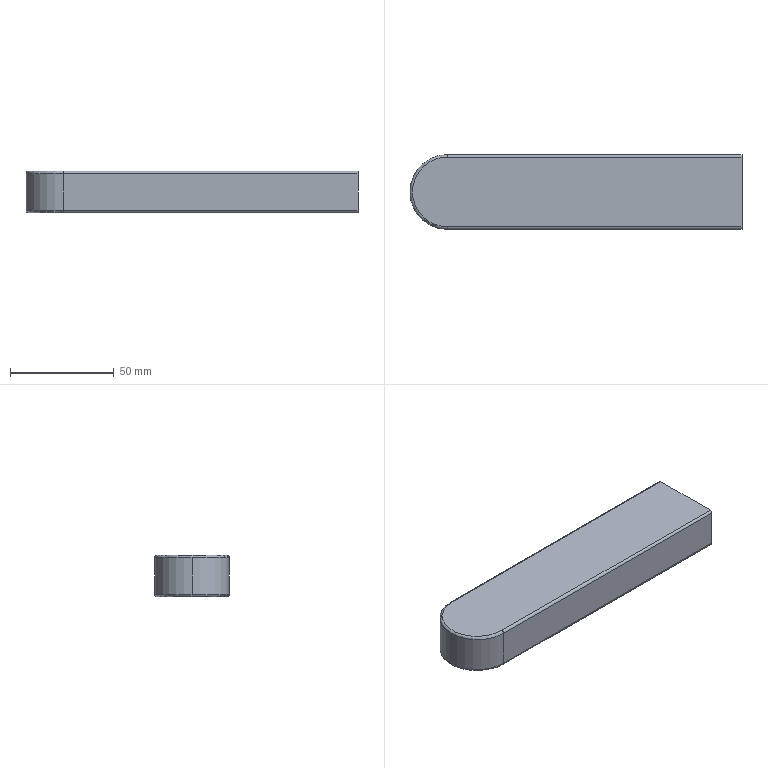Part | SolidWorks | features Extrusion 1, Fillet 1 | 1 solid | 13 faces | box 160 x 36 x 20 mm | volume 112209 mm3 | cylinder 6 | plane 5 | torus 2 | commonest cylinder face diameters 2.4 x4 36 x2
STEP:
#1=CARTESIAN_POINT('',(-9.,-18.,18.8));
#2=VERTEX_POINT('',#1);
#3=CARTESIAN_POINT('',(-27.,0.,18.8));
#4=VERTEX_POINT('',#3);
#5=CARTESIAN_POINT('',(-9.,0.,18.8));
#6=DIRECTION('',(0.,0.,-1.));
#7=DIRECTION('',(1.,0.,0.));
#8=AXIS2_PLACEMENT_3D('',#5,#6,#7);
#9=CIRCLE('',#8,18.);
#10=EDGE_CURVE('',#2,#4,#9,.T.);
#11=ORIENTED_EDGE('',*,*,#10,.T.);
#12=CARTESIAN_POINT('',(-27.,0.,1.2));
#13=VERTEX_POINT('',#12);
#14=CARTESIAN_POINT('',(-27.,0.,20.));
#15=DIRECTION('',(0.,0.,-1.));
#16=VECTOR('',#15,1000.);
#17=LINE('',#14,#16);
#18=EDGE_CURVE('',#4,#13,#17,.T.);
#19=ORIENTED_EDGE('',*,*,#18,.T.);
#20=CARTESIAN_POINT('',(-9.,-18.,1.2));
#21=VERTEX_POINT('',#20);
#22=CARTESIAN_POINT('',(-9.,0.,1.2));
#23=DIRECTION('',(0.,0.,1.));
#24=DIRECTION('',(1.,0.,0.));
#25=AXIS2_PLACEMENT_3D('',#22,#23,#24);
#26=CIRCLE('',#25,18.);
#27=EDGE_CURVE('',#13,#21,#26,.T.);
#28=ORIENTED_EDGE('',*,*,#27,.T.);
#29=CARTESIAN_POINT('',(-9.,-18.,20.));
#30=DIRECTION('',(0.,0.,-1.));
#31=VECTOR('',#30,1000.);
#32=LINE('',#29,#31);
#33=EDGE_CURVE('',#2,#21,#32,.T.);
#34=ORIENTED_EDGE('',*,*,#33,.F.);
#35=EDGE_LOOP('',(#11,#19,#28,#34));
#36=FACE_OUTER_BOUND('',#35,.T.);
#37=CARTESIAN_POINT('',(-9.,0.,20.));
#38=DIRECTION('',(0.,0.,-1.));
#39=DIRECTION('',(-1.,0.,0.));
#40=AXIS2_PLACEMENT_3D('',#37,#38,#39);
#41=CYLINDRICAL_SURFACE('',#40,18.);
#42=ADVANCED_FACE('',(#36),#41,.T.);
#43=CARTESIAN_POINT('',(133.,-16.8,20.));
#44=VERTEX_POINT('',#43);
#45=CARTESIAN_POINT('',(133.,16.8,20.));
#46=VERTEX_POINT('',#45);
#47=CARTESIAN_POINT('',(133.,18.,20.));
#48=DIRECTION('',(0.,1.,0.));
#49=VECTOR('',#48,1000.);
#50=LINE('',#47,#49);
#51=EDGE_CURVE('',#44,#46,#50,.T.);
#52=ORIENTED_EDGE('',*,*,#51,.F.);
#53=CARTESIAN_POINT('',(133.,-18.,18.8));
#54=VERTEX_POINT('',#53);
#55=CARTESIAN_POINT('',(133.,-16.8,18.8));
#56=DIRECTION('',(1.,0.,0.));
#57=DIRECTION('',(0.,0.,1.));
#58=AXIS2_PLACEMENT_3D('',#55,#56,#57);
#59=CIRCLE('',#58,1.2);
#60=EDGE_CURVE('',#44,#54,#59,.T.);
#61=ORIENTED_EDGE('',*,*,#60,.T.);
#62=CARTESIAN_POINT('',(133.,-18.,1.2));
#63=VERTEX_POINT('',#62);
#64=CARTESIAN_POINT('',(133.,-18.,20.));
#65=DIRECTION('',(0.,0.,-1.));
#66=VECTOR('',#65,1000.);
#67=LINE('',#64,#66);
#68=EDGE_CURVE('',#54,#63,#67,.T.);
#69=ORIENTED_EDGE('',*,*,#68,.T.);
#70=CARTESIAN_POINT('',(133.,-16.8,0.));
#71=VERTEX_POINT('',#70);
#72=CARTESIAN_POINT('',(133.,-16.8,1.2));
#73=DIRECTION('',(1.,0.,0.));
#74=DIRECTION('',(0.,0.,1.));
#75=AXIS2_PLACEMENT_3D('',#72,#73,#74);
#76=CIRCLE('',#75,1.2);
#77=EDGE_CURVE('',#63,#71,#76,.T.);
#78=ORIENTED_EDGE('',*,*,#77,.T.);
#79=CARTESIAN_POINT('',(133.,16.8,0.));
#80=VERTEX_POINT('',#79);
#81=CARTESIAN_POINT('',(133.,18.,0.));
#82=DIRECTION('',(0.,1.,0.));
#83=VECTOR('',#82,1000.);
#84=LINE('',#81,#83);
#85=EDGE_CURVE('',#71,#80,#84,.T.);
#86=ORIENTED_EDGE('',*,*,#85,.T.);
#87=CARTESIAN_POINT('',(133.,18.,1.2));
#88=VERTEX_POINT('',#87);
#89=CARTESIAN_POINT('',(133.,16.8,1.2));
#90=DIRECTION('',(1.,0.,0.));
#91=DIRECTION('',(0.,0.,1.));
#92=AXIS2_PLACEMENT_3D('',#89,#90,#91);
#93=CIRCLE('',#92,1.2);
#94=EDGE_CURVE('',#80,#88,#93,.T.);
#95=ORIENTED_EDGE('',*,*,#94,.T.);
#96=CARTESIAN_POINT('',(133.,18.,18.8));
#97=VERTEX_POINT('',#96);
#98=CARTESIAN_POINT('',(133.,18.,20.));
#99=DIRECTION('',(0.,0.,-1.));
#100=VECTOR('',#99,1000.);
#101=LINE('',#98,#100);
#102=EDGE_CURVE('',#97,#88,#101,.T.);
#103=ORIENTED_EDGE('',*,*,#102,.F.);
#104=CARTESIAN_POINT('',(133.,16.8,18.8));
#105=DIRECTION('',(1.,0.,0.));
#106=DIRECTION('',(0.,0.,1.));
#107=AXIS2_PLACEMENT_3D('',#104,#105,#106);
#108=CIRCLE('',#107,1.2);
#109=EDGE_CURVE('',#97,#46,#108,.T.);
#110=ORIENTED_EDGE('',*,*,#109,.T.);
#111=EDGE_LOOP('',(#52,#61,#69,#78,#86,#95,#103,#110));
#112=FACE_OUTER_BOUND('',#111,.T.);
#113=CARTESIAN_POINT('',(133.,18.,20.));
#114=DIRECTION('',(-1.,0.,0.));
#115=DIRECTION('',(0.,0.,1.));
#116=AXIS2_PLACEMENT_3D('',#113,#114,#115);
#117=PLANE('',#116);
#118=ADVANCED_FACE('',(#112),#117,.F.);
#119=CARTESIAN_POINT('',(-9.,18.,18.8));
#120=VERTEX_POINT('',#119);
#121=CARTESIAN_POINT('',(-9.,18.,1.2));
#122=VERTEX_POINT('',#121);
#123=CARTESIAN_POINT('',(-9.,18.,20.));
#124=DIRECTION('',(0.,0.,-1.));
#125=VECTOR('',#124,1000.);
#126=LINE('',#123,#125);
#127=EDGE_CURVE('',#120,#122,#126,.T.);
#128=ORIENTED_EDGE('',*,*,#127,.F.);
#129=CARTESIAN_POINT('',(133.,18.,18.8));
#130=DIRECTION('',(1.,0.,0.));
#131=VECTOR('',#130,1000.);
#132=LINE('',#129,#131);
#133=EDGE_CURVE('',#120,#97,#132,.T.);
#134=ORIENTED_EDGE('',*,*,#133,.T.);
#135=ORIENTED_EDGE('',*,*,#102,.T.);
#136=CARTESIAN_POINT('',(-9.,18.,1.2));
#137=DIRECTION('',(-1.,0.,0.));
#138=VECTOR('',#137,1000.);
#139=LINE('',#136,#138);
#140=EDGE_CURVE('',#88,#122,#139,.T.);
#141=ORIENTED_EDGE('',*,*,#140,.T.);
#142=EDGE_LOOP('',(#128,#134,#135,#141));
#143=FACE_OUTER_BOUND('',#142,.T.);
#144=CARTESIAN_POINT('',(-9.,18.,20.));
#145=DIRECTION('',(0.,-1.,0.));
#146=DIRECTION('',(0.,0.,-1.));
#147=AXIS2_PLACEMENT_3D('',#144,#145,#146);
#148=PLANE('',#147);
#149=ADVANCED_FACE('',(#143),#148,.F.);
#150=ORIENTED_EDGE('',*,*,#18,.F.);
#151=CARTESIAN_POINT('',(-9.,0.,18.8));
#152=DIRECTION('',(0.,0.,-1.));
#153=DIRECTION('',(1.,0.,0.));
#154=AXIS2_PLACEMENT_3D('',#151,#152,#153);
#155=CIRCLE('',#154,18.);
#156=EDGE_CURVE('',#4,#120,#155,.T.);
#157=ORIENTED_EDGE('',*,*,#156,.T.);
#158=ORIENTED_EDGE('',*,*,#127,.T.);
#159=CARTESIAN_POINT('',(-9.,0.,1.2));
#160=DIRECTION('',(0.,0.,1.));
#161=DIRECTION('',(1.,0.,0.));
#162=AXIS2_PLACEMENT_3D('',#159,#160,#161);
#163=CIRCLE('',#162,18.);
#164=EDGE_CURVE('',#122,#13,#163,.T.);
#165=ORIENTED_EDGE('',*,*,#164,.T.);
#166=EDGE_LOOP('',(#150,#157,#158,#165));
#167=FACE_OUTER_BOUND('',#166,.T.);
#168=CARTESIAN_POINT('',(-9.,0.,20.));
#169=DIRECTION('',(0.,0.,-1.));
#170=DIRECTION('',(-1.,0.,0.));
#171=AXIS2_PLACEMENT_3D('',#168,#169,#170);
#172=CYLINDRICAL_SURFACE('',#171,18.);
#173=ADVANCED_FACE('',(#167),#172,.T.);
#174=ORIENTED_EDGE('',*,*,#68,.F.);
#175=CARTESIAN_POINT('',(-9.,-18.,18.8));
#176=DIRECTION('',(-1.,0.,0.));
#177=VECTOR('',#176,1000.);
#178=LINE('',#175,#177);
#179=EDGE_CURVE('',#54,#2,#178,.T.);
#180=ORIENTED_EDGE('',*,*,#179,.T.);
#181=ORIENTED_EDGE('',*,*,#33,.T.);
#182=CARTESIAN_POINT('',(-9.,-18.,1.2));
#183=DIRECTION('',(1.,0.,0.));
#184=VECTOR('',#183,1000.);
#185=LINE('',#182,#184);
#186=EDGE_CURVE('',#21,#63,#185,.T.);
#187=ORIENTED_EDGE('',*,*,#186,.T.);
#188=EDGE_LOOP('',(#174,#180,#181,#187));
#189=FACE_OUTER_BOUND('',#188,.T.);
#190=CARTESIAN_POINT('',(-9.,-18.,20.));
#191=DIRECTION('',(0.,1.,0.));
#192=DIRECTION('',(0.,0.,1.));
#193=AXIS2_PLACEMENT_3D('',#190,#191,#192);
#194=PLANE('',#193);
#195=ADVANCED_FACE('',(#189),#194,.F.);
#196=CARTESIAN_POINT('',(-9.,16.8,20.));
#197=VERTEX_POINT('',#196);
#198=CARTESIAN_POINT('',(-9.,-16.8,20.));
#199=VERTEX_POINT('',#198);
#200=CARTESIAN_POINT('',(-9.,0.,20.));
#201=DIRECTION('',(0.,0.,1.));
#202=DIRECTION('',(1.,0.,0.));
#203=AXIS2_PLACEMENT_3D('',#200,#201,#202);
#204=CIRCLE('',#203,16.8);
#205=EDGE_CURVE('',#197,#199,#204,.T.);
#206=ORIENTED_EDGE('',*,*,#205,.T.);
#207=CARTESIAN_POINT('',(133.,-16.8,20.));
#208=DIRECTION('',(1.,0.,0.));
#209=VECTOR('',#208,1000.);
#210=LINE('',#207,#209);
#211=EDGE_CURVE('',#199,#44,#210,.T.);
#212=ORIENTED_EDGE('',*,*,#211,.T.);
#213=ORIENTED_EDGE('',*,*,#51,.T.);
#214=CARTESIAN_POINT('',(-9.,16.8,20.));
#215=DIRECTION('',(-1.,0.,0.));
#216=VECTOR('',#215,1000.);
#217=LINE('',#214,#216);
#218=EDGE_CURVE('',#46,#197,#217,.T.);
#219=ORIENTED_EDGE('',*,*,#218,.T.);
#220=EDGE_LOOP('',(#206,#212,#213,#219));
#221=FACE_OUTER_BOUND('',#220,.T.);
#222=CARTESIAN_POINT('',(-9.,0.,20.));
#223=DIRECTION('',(0.,0.,1.));
#224=DIRECTION('',(1.,0.,0.));
#225=AXIS2_PLACEMENT_3D('',#222,#223,#224);
#226=PLANE('',#225);
#227=ADVANCED_FACE('',(#221),#226,.T.);
#228=CARTESIAN_POINT('',(-9.,-16.8,0.));
#229=VERTEX_POINT('',#228);
#230=CARTESIAN_POINT('',(-9.,16.8,0.));
#231=VERTEX_POINT('',#230);
#232=CARTESIAN_POINT('',(-9.,0.,0.));
#233=DIRECTION('',(0.,0.,-1.));
#234=DIRECTION('',(1.,0.,0.));
#235=AXIS2_PLACEMENT_3D('',#232,#233,#234);
#236=CIRCLE('',#235,16.8);
#237=EDGE_CURVE('',#229,#231,#236,.T.);
#238=ORIENTED_EDGE('',*,*,#237,.T.);
#239=CARTESIAN_POINT('',(-9.,16.8,0.));
#240=DIRECTION('',(1.,0.,0.));
#241=VECTOR('',#240,1000.);
#242=LINE('',#239,#241);
#243=EDGE_CURVE('',#231,#80,#242,.T.);
#244=ORIENTED_EDGE('',*,*,#243,.T.);
#245=ORIENTED_EDGE('',*,*,#85,.F.);
#246=CARTESIAN_POINT('',(-9.,-16.8,0.));
#247=DIRECTION('',(-1.,0.,0.));
#248=VECTOR('',#247,1000.);
#249=LINE('',#246,#248);
#250=EDGE_CURVE('',#71,#229,#249,.T.);
#251=ORIENTED_EDGE('',*,*,#250,.T.);
#252=EDGE_LOOP('',(#238,#244,#245,#251));
#253=FACE_OUTER_BOUND('',#252,.T.);
#254=CARTESIAN_POINT('',(-9.,0.,0.));
#255=DIRECTION('',(0.,0.,1.));
#256=DIRECTION('',(1.,0.,0.));
#257=AXIS2_PLACEMENT_3D('',#254,#255,#256);
#258=PLANE('',#257);
#259=ADVANCED_FACE('',(#253),#258,.F.);
#260=ORIENTED_EDGE('',*,*,#109,.F.);
#261=ORIENTED_EDGE('',*,*,#133,.F.);
#262=CARTESIAN_POINT('',(-9.,16.8,18.8));
#263=DIRECTION('',(-1.,0.,0.));
#264=DIRECTION('',(0.,0.,1.));
#265=AXIS2_PLACEMENT_3D('',#262,#263,#264);
#266=CIRCLE('',#265,1.2);
#267=EDGE_CURVE('',#197,#120,#266,.T.);
#268=ORIENTED_EDGE('',*,*,#267,.F.);
#269=ORIENTED_EDGE('',*,*,#218,.F.);
#270=EDGE_LOOP('',(#260,#261,#268,#269));
#271=FACE_OUTER_BOUND('',#270,.T.);
#272=CARTESIAN_POINT('',(-9.,16.8,18.8));
#273=DIRECTION('',(1.,0.,0.));
#274=DIRECTION('',(0.,0.,-1.));
#275=AXIS2_PLACEMENT_3D('',#272,#273,#274);
#276=CYLINDRICAL_SURFACE('',#275,1.2);
#277=ADVANCED_FACE('',(#271),#276,.T.);
#278=ORIENTED_EDGE('',*,*,#267,.T.);
#279=ORIENTED_EDGE('',*,*,#156,.F.);
#280=ORIENTED_EDGE('',*,*,#10,.F.);
#281=CARTESIAN_POINT('',(-9.,-16.8,18.8));
#282=DIRECTION('',(1.,0.,0.));
#283=DIRECTION('',(0.,0.,-1.));
#284=AXIS2_PLACEMENT_3D('',#281,#282,#283);
#285=CIRCLE('',#284,1.2);
#286=EDGE_CURVE('',#199,#2,#285,.T.);
#287=ORIENTED_EDGE('',*,*,#286,.F.);
#288=ORIENTED_EDGE('',*,*,#205,.F.);
#289=EDGE_LOOP('',(#278,#279,#280,#287,#288));
#290=FACE_OUTER_BOUND('',#289,.T.);
#291=CARTESIAN_POINT('',(-9.,0.,18.8));
#292=DIRECTION('',(0.,0.,1.));
#293=DIRECTION('',(1.,0.,0.));
#294=AXIS2_PLACEMENT_3D('',#291,#292,#293);
#295=TOROIDAL_SURFACE('',#294,16.8,1.2);
#296=ADVANCED_FACE('',(#290),#295,.T.);
#297=ORIENTED_EDGE('',*,*,#286,.T.);
#298=ORIENTED_EDGE('',*,*,#179,.F.);
#299=ORIENTED_EDGE('',*,*,#60,.F.);
#300=ORIENTED_EDGE('',*,*,#211,.F.);
#301=EDGE_LOOP('',(#297,#298,#299,#300));
#302=FACE_OUTER_BOUND('',#301,.T.);
#303=CARTESIAN_POINT('',(-9.,-16.8,18.8));
#304=DIRECTION('',(-1.,0.,0.));
#305=DIRECTION('',(0.,0.,1.));
#306=AXIS2_PLACEMENT_3D('',#303,#304,#305);
#307=CYLINDRICAL_SURFACE('',#306,1.2);
#308=ADVANCED_FACE('',(#302),#307,.T.);
#309=ORIENTED_EDGE('',*,*,#77,.F.);
#310=ORIENTED_EDGE('',*,*,#186,.F.);
#311=CARTESIAN_POINT('',(-9.,-16.8,1.2));
#312=DIRECTION('',(-1.,0.,0.));
#313=DIRECTION('',(0.,0.,1.));
#314=AXIS2_PLACEMENT_3D('',#311,#312,#313);
#315=CIRCLE('',#314,1.2);
#316=EDGE_CURVE('',#229,#21,#315,.T.);
#317=ORIENTED_EDGE('',*,*,#316,.F.);
#318=ORIENTED_EDGE('',*,*,#250,.F.);
#319=EDGE_LOOP('',(#309,#310,#317,#318));
#320=FACE_OUTER_BOUND('',#319,.T.);
#321=CARTESIAN_POINT('',(-9.,-16.8,1.2));
#322=DIRECTION('',(1.,0.,0.));
#323=DIRECTION('',(0.,0.,-1.));
#324=AXIS2_PLACEMENT_3D('',#321,#322,#323);
#325=CYLINDRICAL_SURFACE('',#324,1.2);
#326=ADVANCED_FACE('',(#320),#325,.T.);
#327=ORIENTED_EDGE('',*,*,#316,.T.);
#328=ORIENTED_EDGE('',*,*,#27,.F.);
#329=ORIENTED_EDGE('',*,*,#164,.F.);
#330=CARTESIAN_POINT('',(-9.,16.8,1.2));
#331=DIRECTION('',(1.,0.,0.));
#332=DIRECTION('',(0.,0.,-1.));
#333=AXIS2_PLACEMENT_3D('',#330,#331,#332);
#334=CIRCLE('',#333,1.2);
#335=EDGE_CURVE('',#231,#122,#334,.T.);
#336=ORIENTED_EDGE('',*,*,#335,.F.);
#337=ORIENTED_EDGE('',*,*,#237,.F.);
#338=EDGE_LOOP('',(#327,#328,#329,#336,#337));
#339=FACE_OUTER_BOUND('',#338,.T.);
#340=CARTESIAN_POINT('',(-9.,0.,1.2));
#341=DIRECTION('',(0.,0.,1.));
#342=DIRECTION('',(1.,0.,0.));
#343=AXIS2_PLACEMENT_3D('',#340,#341,#342);
#344=TOROIDAL_SURFACE('',#343,16.8,1.2);
#345=ADVANCED_FACE('',(#339),#344,.T.);
#346=ORIENTED_EDGE('',*,*,#94,.F.);
#347=ORIENTED_EDGE('',*,*,#243,.F.);
#348=ORIENTED_EDGE('',*,*,#335,.T.);
#349=ORIENTED_EDGE('',*,*,#140,.F.);
#350=EDGE_LOOP('',(#346,#347,#348,#349));
#351=FACE_OUTER_BOUND('',#350,.T.);
#352=CARTESIAN_POINT('',(-9.,16.8,1.2));
#353=DIRECTION('',(-1.,0.,0.));
#354=DIRECTION('',(0.,0.,1.));
#355=AXIS2_PLACEMENT_3D('',#352,#353,#354);
#356=CYLINDRICAL_SURFACE('',#355,1.2);
#357=ADVANCED_FACE('',(#351),#356,.T.);
#358=CLOSED_SHELL('',(#42,#118,#149,#173,#195,#227,#259,#277,#296,#308,#326,#345,#357));
#359=MANIFOLD_SOLID_BREP('',#358);
#360=CARTESIAN_POINT('',(0.,0.,0.));
#361=DIRECTION('',(0.,0.,1.));
#362=DIRECTION('',(1.,0.,0.));
#363=AXIS2_PLACEMENT_3D('',#360,#361,#362);
#364=(LENGTH_UNIT()NAMED_UNIT(*)SI_UNIT(.MILLI.,.METRE.));
#365=UNCERTAINTY_MEASURE_WITH_UNIT(LENGTH_MEASURE(0.00001),#364,'','');
#366=(NAMED_UNIT(*)PLANE_ANGLE_UNIT()SI_UNIT($,.RADIAN.));
#367=(NAMED_UNIT(*)SI_UNIT($,.STERADIAN.)SOLID_ANGLE_UNIT());
#368=(GEOMETRIC_REPRESENTATION_CONTEXT(3)GLOBAL_UNCERTAINTY_ASSIGNED_CONTEXT((#365))GLOBAL_UNIT_ASSIGNED_CONTEXT((#364,#366,#367))REPRESENTATION_CONTEXT('',''));
#369=ADVANCED_BREP_SHAPE_REPRESENTATION('',(#359,#363),#368);